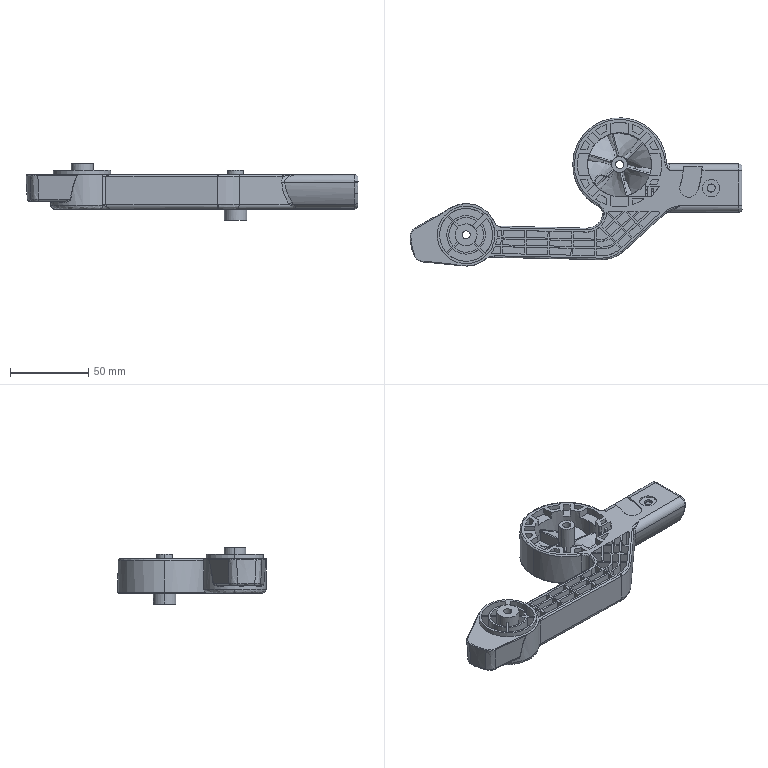Part | SolidWorks | features BaseBody 1 | 1 solid | 661 faces | box 212.741 x 95 x 36 mm | volume 90575 mm3 | plane 300 | spline 178 | cylinder 176 | torus 4 | cone 3 | commonest cylinder face diameters 37 x15 1 x12 54 x10 2 x9 4 x9 46 x7